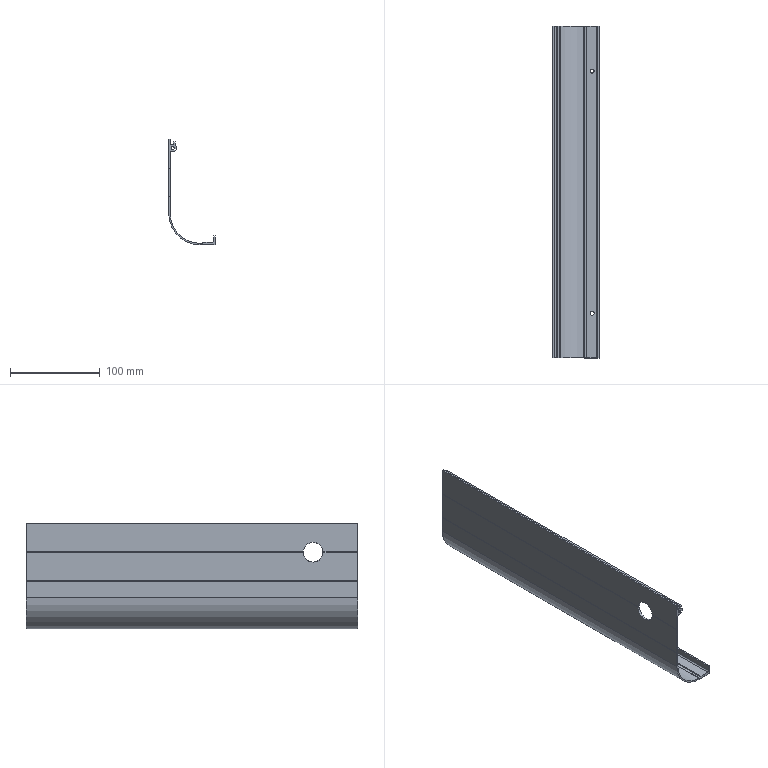Part | STEP file | 601-10-0092 | 1 solid | 70 faces | box 52 x 370 x 118 mm | volume 126535 mm3 | plane 34 | cylinder 26 | cone 10 | commonest cylinder face diameters 3.3 x6 4.5 x4 3.2 x3 8 x3 1 x2 22 x2